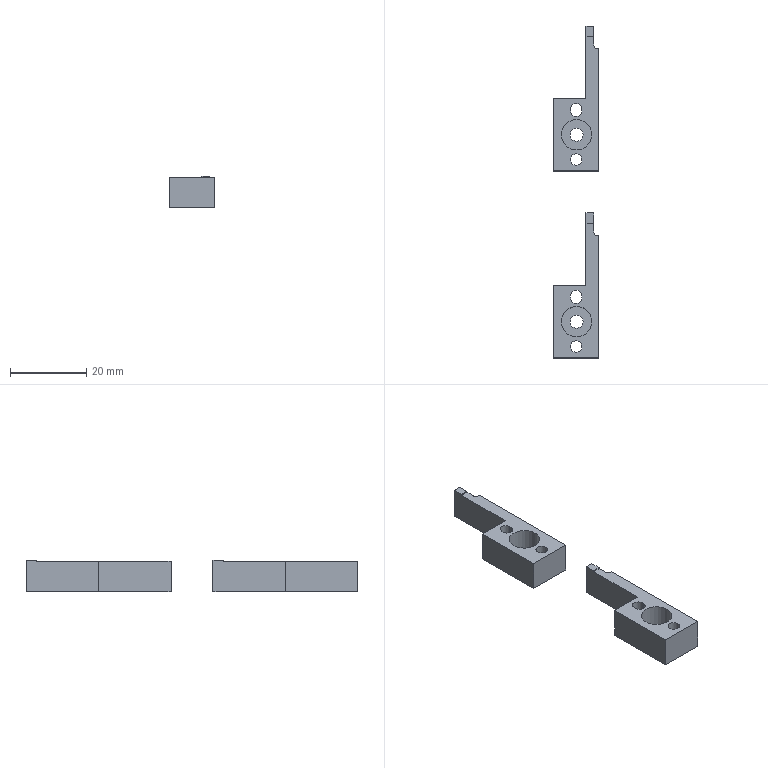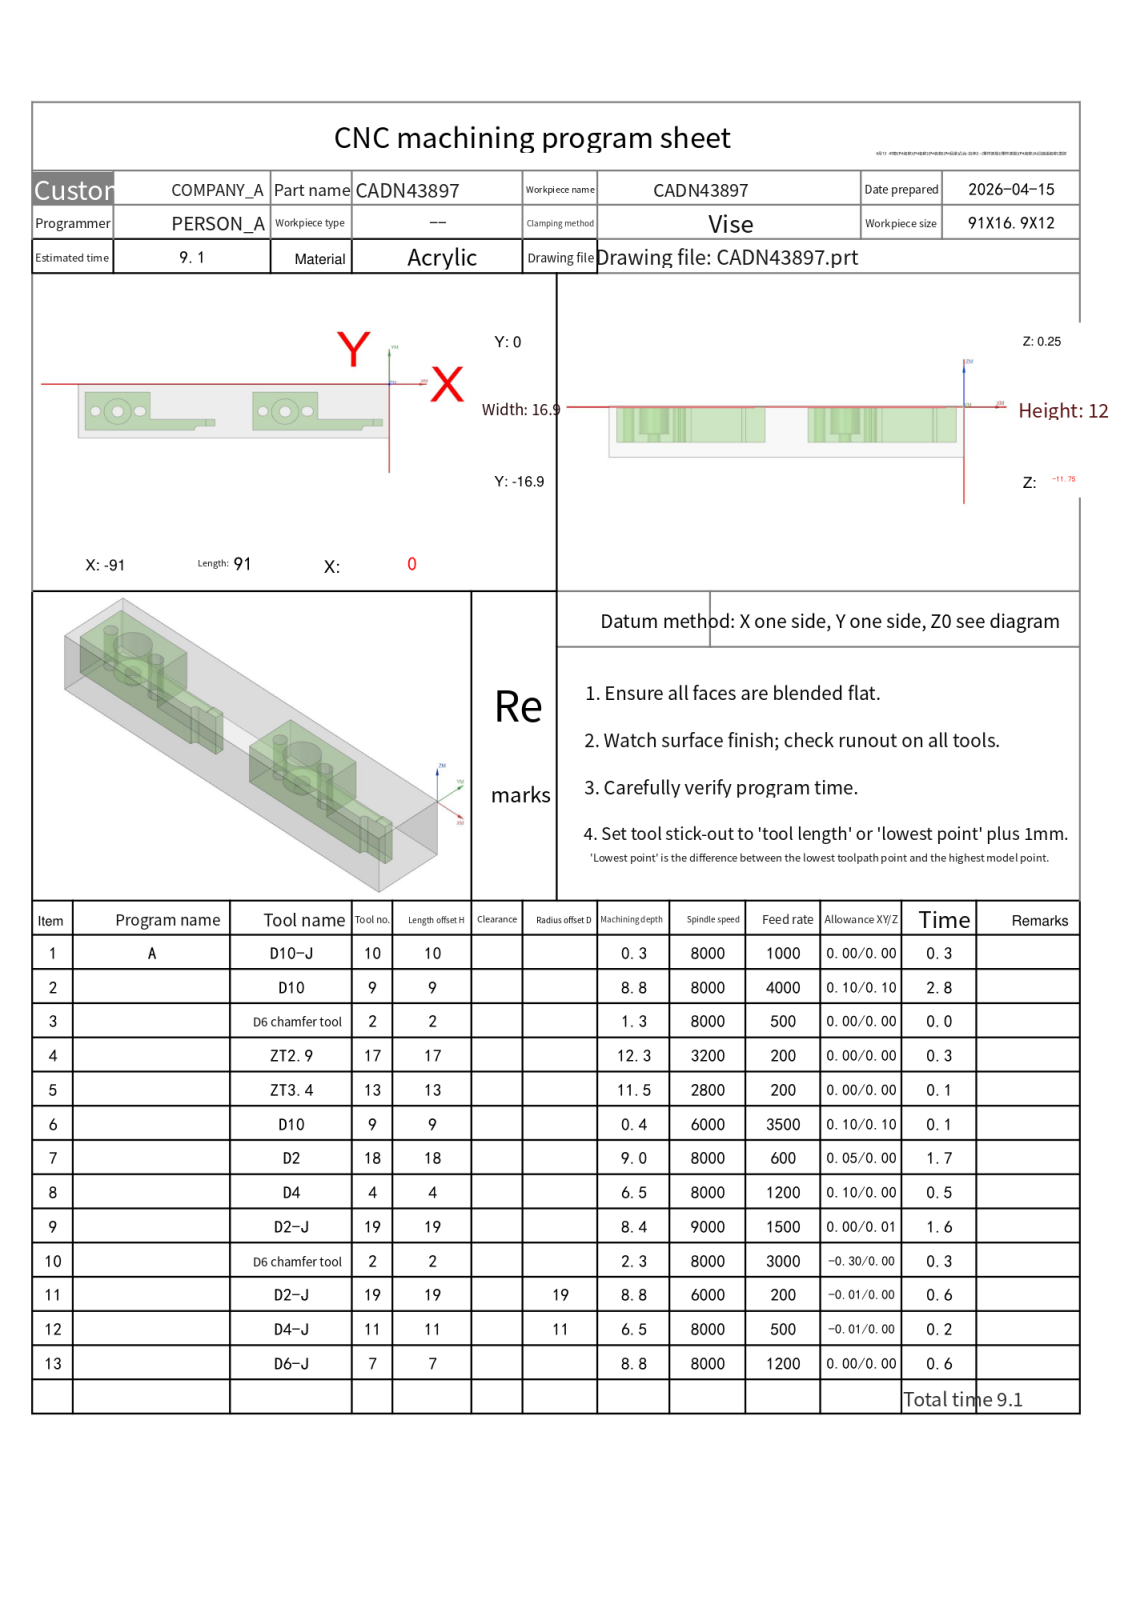NC program | NX | posted by the shop | part box 11.9 x 87 x 8.25 mm
Lines 1 to 2110 of 9110, first 1642 of 2108 lines:
%
O0001
(Machine time: 11.64 MIN)
(===Total Tool:10===)
(T10=D10-J  D=10.  R=0.   D-  H10 Z=-0.   )
(T9=D10     D=10.  R=0.   D-  H09 Z=-8.55 )
(T2=D6 chamfer tool   D=6.   R=0.   D-  H02 Z=-2.05 )
(T17=ZT2.9  D=2.9  DR_a=120 D-  H17 Z=-12.09)
(T13=ZT3.4  D=3.4  DR_a=118 D-  H13 Z=-11.27)
(T18=D2     D=2.   R=0.   D-  H18 Z=-8.75 )
(T4=D4      D=4.   R=0.   D-  H04 Z=-6.25 )
(T19=D2-J   D=2.   R=0.   D-  H19 Z=-8.55 )
(T11=D4-J   D=4.   R=0.   D11 H11 Z=-6.25 )
(T7=D6-J    D=6.   R=0.   D7  H07 Z=-8.55 )
G80 G90 G17 G49 G40
G91 G28 Z0
M01
N1 T10 M06
(D10-J  D=10. R=0. H=10 ce=0.00 di=0.00)
G00 G90 G54 X-99. Y-2.975 M03 S8000
G43 H10 Z20.
M08
Z2.
G01 Z0.0 F1000.
X-94.
X3.
Y-8.45
X-94.
Y-13.925
X3.
X8.
Z2.
G00 Z20.
G91 G28 Z0.0
M05
M09
G91 G28 Z0.0
M01
N2 T09 M06
(D10  D=10. R=0. H=09 ce=0.10 di=0.10)
G00 G90 G54 X-62.25 Y12. M03 S8000
G43 H09 Z10.25
M08
Z.725
G01 Z-.475 F4000.
Y7.5
G03 X-55.25 Y.5 I7. J0.0
G01 X-45.766
G02 X-40. Y4. I5.766 J-3.
G01 X-21.
G02 X-15.234 Y.5 I0.0 J-6.5
G01 X0.0
G02 X.5 Y0.0 I0.0 J-.5
G01 Y-4.341
G02 X-.5 Y-5.341 I-1. J0.0
X-.786 Y-5.299 I0.0 J1.
G01 X-3.474 Y-4.498
G03 X-3.76 Y-4.456 I-.285 J-.958
X-4.126 Y-4.526 I0.0 J-1.
G01 X-4.199 Y-4.54
X-14.301
G02 X-14.5 Y-4.341 I.001 J.2
G01 Y-4.199
G02 X-14.301 Y-4. I.2 J-.001
G01 X-4.199
X-4.121 Y-4.016
G03 X-3.726 Y-4.098 I.395 J.919
X-3.48 Y-4.067 I0.0 J1.
G01 X-.746 Y-3.372
G02 X-.5 Y-3.341 I.246 J-.969
X.5 Y-4.341 I0.0 J-1.
G01 Y-5.04
G02 X4.5 Y-11.04 I-2.5 J-6.
G01 Y-13.1
G02 X-2. Y-19.6 I-6.5 J0.0
G01 X-4.1
G02 X-8. Y-20.9 I-3.9 J5.2
G01 X-40.
G02 X-45.766 Y-17.4 I0.0 J6.5
G01 X-46.126
G02 X-51. Y-19.6 I-4.874 J4.3
G01 X-53.1
G02 X-57. Y-20.9 I-3.9 J5.2
G01 X-89.
G02 X-95.5 Y-14.4 I0.0 J6.5
G01 Y-2.5
G02 X-89. Y4. I6.5 J0.0
G01 X-70.
G02 X-64.234 Y.5 I0.0 J-6.5
G01 X-50.25
G02 X-49.26 Y-.357 I0.0 J-1.
G01 X-48.912 Y-2.774
G03 X-47.496 Y-4. I1.416 J.204
G01 X-47.198
G02 X-46.513 Y-4.568 I-.002 J-.7
G03 X-46.082 Y-5.125 I.765 J.147
G01 X-45.7 Y-5.306
X-45.52 Y-5.346
G03 X-45.1 Y-4.926 I0.0 J.42
G01 Y-2.5
G02 X-40. Y2.6 I5.1 J0.0
G01 X-21.
G02 X-15.9 Y-2.5 I0.0 J-5.1
G01 Y-5.94
X-2.
G02 X3.1 Y-11.04 I0.0 J-5.1
G01 Y-13.1
G02 X-2. Y-18.2 I-5.1 J0.0
G01 X-4.599
G02 X-8. Y-19.5 I-3.401 J3.8
G01 X-40.
G02 X-45.1 Y-14.4 I0.0 J5.1
G01 Y-4.926
G03 X-45.52 Y-4.506 I-.42 J0.0
G01 X-45.7 Y-4.547
X-46.306 Y-4.834
G03 X-46.522 Y-5.097 I.172 J-.361
G02 X-47.2 Y-5.624 I-.678 J.172
X-47.568 Y-5.52 I0.0 J.7
G03 X-51. Y-4.54 I-3.432 J-5.52
G01 X-63.301
G02 X-63.481 Y-4.425 I.001 J.2
G03 X-63.892 Y-4.013 I-.783 J-.37
G01 X-64.3 Y-3.819
X-64.48 Y-3.779
G03 X-64.9 Y-4.199 I0.0 J-.42
G01 Y-5.94
X-51.
G02 X-45.9 Y-11.04 I0.0 J-5.1
G01 Y-13.1
G02 X-51. Y-18.2 I-5.1 J0.0
G01 X-53.599
G02 X-57. Y-19.5 I-3.401 J3.8
G01 X-89.
G02 X-94.1 Y-14.4 I0.0 J5.1
G01 Y-2.5
G02 X-89. Y2.6 I5.1 J0.0
G01 X-70.
G02 X-64.9 Y-2.5 I0.0 J-5.1
G01 Y-4.199
G03 X-64.48 Y-4.619 I.42 J0.0
G01 X-64.3 Y-4.578
X-63.654 Y-4.272
G03 X-63.475 Y-4.104 I-.172 J.361
G02 X-63.301 Y-4. I.175 J-.096
G01 X-50.25
X-49.75
G03 X-46.25 Y-.5 I0.0 J3.5
G01 Y12.
Z.725
G00 Z3.
G01 X-62.25 F6000.
G00 Z.25
G01 Z-.95 F4000.
Y7.5
G03 X-55.25 Y.5 I7. J0.0
G01 X-45.766
G02 X-40. Y4. I5.766 J-3.
G01 X-21.
G02 X-15.234 Y.5 I0.0 J-6.5
G01 X0.0
G02 X.5 Y0.0 I0.0 J-.5
G01 Y-4.341
G02 X-.5 Y-5.341 I-1. J0.0
X-.786 Y-5.299 I0.0 J1.
G01 X-3.474 Y-4.498
G03 X-3.759 Y-4.456 I-.285 J-.958
X-4.126 Y-4.526 I0.0 J-1.
G01 X-4.199 Y-4.54
X-14.301
G02 X-14.5 Y-4.341 I.001 J.2
G01 Y-4.199
G02 X-14.301 Y-4. I.2 J-.001
G01 X-4.199
X-4.121 Y-4.016
G03 X-3.726 Y-4.098 I.395 J.919
X-3.48 Y-4.067 I0.0 J1.
G01 X-.746 Y-3.372
G02 X-.5 Y-3.341 I.246 J-.969
X.5 Y-4.341 I0.0 J-1.
G01 Y-5.04
G02 X4.5 Y-11.04 I-2.5 J-6.
G01 Y-13.1
G02 X-2. Y-19.6 I-6.5 J0.0
G01 X-4.1
G02 X-8. Y-20.9 I-3.9 J5.2
G01 X-40.
G02 X-45.766 Y-17.4 I0.0 J6.5
G01 X-46.126
G02 X-51. Y-19.6 I-4.874 J4.3
G01 X-53.1
G02 X-57. Y-20.9 I-3.9 J5.2
G01 X-89.
G02 X-95.5 Y-14.4 I0.0 J6.5
G01 Y-2.5
G02 X-89. Y4. I6.5 J0.0
G01 X-70.
G02 X-64.234 Y.5 I0.0 J-6.5
G01 X-50.25
G02 X-49.26 Y-.357 I0.0 J-1.
G01 X-48.912 Y-2.774
G03 X-47.496 Y-4. I1.416 J.204
G01 X-47.198
G02 X-46.513 Y-4.568 I-.002 J-.7
G03 X-46.082 Y-5.125 I.765 J.147
G01 X-45.7 Y-5.306
X-45.52 Y-5.346
G03 X-45.1 Y-4.926 I0.0 J.42
G01 Y-2.5
G02 X-40. Y2.6 I5.1 J0.0
G01 X-21.
G02 X-15.9 Y-2.5 I0.0 J-5.1
G01 Y-5.94
X-2.
G02 X3.1 Y-11.04 I0.0 J-5.1
G01 Y-13.1
G02 X-2. Y-18.2 I-5.1 J0.0
G01 X-4.599
G02 X-8. Y-19.5 I-3.401 J3.8
G01 X-40.
G02 X-45.1 Y-14.4 I0.0 J5.1
G01 Y-4.926
G03 X-45.52 Y-4.506 I-.42 J0.0
G01 X-45.7 Y-4.547
X-46.305 Y-4.834
G03 X-46.521 Y-5.097 I.172 J-.361
G02 X-47.2 Y-5.624 I-.678 J.172
X-47.568 Y-5.52 I0.0 J.7
G03 X-51. Y-4.54 I-3.432 J-5.52
G01 X-63.301
G02 X-63.481 Y-4.425 I.001 J.2
G03 X-63.892 Y-4.013 I-.783 J-.37
G01 X-64.3 Y-3.82
X-64.48 Y-3.779
G03 X-64.9 Y-4.199 I0.0 J-.42
G01 Y-5.94
X-51.
G02 X-45.9 Y-11.04 I0.0 J-5.1
G01 Y-13.1
G02 X-51. Y-18.2 I-5.1 J0.0
G01 X-53.599
G02 X-57. Y-19.5 I-3.401 J3.8
G01 X-89.
G02 X-94.1 Y-14.4 I0.0 J5.1
G01 Y-2.5
G02 X-89. Y2.6 I5.1 J0.0
G01 X-70.
G02 X-64.9 Y-2.5 I0.0 J-5.1
G01 Y-4.199
G03 X-64.48 Y-4.619 I.42 J0.0
G01 X-64.3 Y-4.579
X-63.654 Y-4.272
G03 X-63.475 Y-4.104 I-.172 J.361
G02 X-63.301 Y-4. I.175 J-.096
G01 X-50.25
X-49.75
G03 X-46.25 Y-.5 I0.0 J3.5
G01 Y12.
Z.25
G00 Z2.525
G01 X-62.25 F6000.
G00 Z-.225
G01 Z-1.425 F4000.
Y7.5
G03 X-55.25 Y.5 I7. J0.0
G01 X-45.766
G02 X-40. Y4. I5.766 J-3.
G01 X-21.
G02 X-15.234 Y.5 I0.0 J-6.5
G01 X0.0
G02 X.5 Y0.0 I0.0 J-.5
G01 Y-4.341
G02 X-.5 Y-5.341 I-1. J0.0
X-.786 Y-5.299 I0.0 J1.
G01 X-3.474 Y-4.498
G03 X-3.76 Y-4.456 I-.285 J-.958
X-4.126 Y-4.526 I0.0 J-1.
G01 X-4.199 Y-4.54
X-14.301
G02 X-14.5 Y-4.341 I.001 J.2
G01 Y-4.199
G02 X-14.301 Y-4. I.2 J-.001
G01 X-4.199
X-4.121 Y-4.016
G03 X-3.726 Y-4.098 I.395 J.919
X-3.48 Y-4.067 I0.0 J1.
G01 X-.746 Y-3.372
G02 X-.5 Y-3.341 I.246 J-.969
X.5 Y-4.341 I0.0 J-1.
G01 Y-5.04
G02 X4.5 Y-11.04 I-2.5 J-6.
G01 Y-13.1
G02 X-2. Y-19.6 I-6.5 J0.0
G01 X-4.1
G02 X-8. Y-20.9 I-3.9 J5.2
G01 X-40.
G02 X-45.766 Y-17.4 I0.0 J6.5
G01 X-46.126
G02 X-51. Y-19.6 I-4.874 J4.3
G01 X-53.1
G02 X-57. Y-20.9 I-3.9 J5.2
G01 X-89.
G02 X-95.5 Y-14.4 I0.0 J6.5
G01 Y-2.5
G02 X-89. Y4. I6.5 J0.0
G01 X-70.
G02 X-64.234 Y.5 I0.0 J-6.5
G01 X-50.25
G02 X-49.26 Y-.357 I0.0 J-1.
G01 X-48.912 Y-2.774
G03 X-47.496 Y-4. I1.416 J.204
G01 X-47.198
G02 X-46.513 Y-4.568 I-.002 J-.7
G03 X-46.082 Y-5.125 I.765 J.147
G01 X-45.7 Y-5.306
X-45.52 Y-5.346
G03 X-45.1 Y-4.926 I0.0 J.42
G01 Y-2.5
G02 X-40. Y2.6 I5.1 J0.0
G01 X-21.
G02 X-15.9 Y-2.5 I0.0 J-5.1
G01 Y-5.94
X-2.
G02 X3.1 Y-11.04 I0.0 J-5.1
G01 Y-13.1
G02 X-2. Y-18.2 I-5.1 J0.0
G01 X-4.599
G02 X-8. Y-19.5 I-3.401 J3.8
G01 X-40.
G02 X-45.1 Y-14.4 I0.0 J5.1
G01 Y-4.926
G03 X-45.52 Y-4.506 I-.42 J0.0
G01 X-45.7 Y-4.547
X-46.306 Y-4.834
G03 X-46.522 Y-5.097 I.172 J-.361
G02 X-47.2 Y-5.624 I-.678 J.172
X-47.568 Y-5.52 I0.0 J.7
G03 X-51. Y-4.54 I-3.432 J-5.52
G01 X-63.301
G02 X-63.481 Y-4.425 I.001 J.2
G03 X-63.892 Y-4.013 I-.783 J-.37
G01 X-64.3 Y-3.819
X-64.48 Y-3.779
G03 X-64.9 Y-4.199 I0.0 J-.42
G01 Y-5.94
X-51.
G02 X-45.9 Y-11.04 I0.0 J-5.1
G01 Y-13.1
G02 X-51. Y-18.2 I-5.1 J0.0
G01 X-53.599
G02 X-57. Y-19.5 I-3.401 J3.8
G01 X-89.
G02 X-94.1 Y-14.4 I0.0 J5.1
G01 Y-2.5
G02 X-89. Y2.6 I5.1 J0.0
G01 X-70.
G02 X-64.9 Y-2.5 I0.0 J-5.1
G01 Y-4.199
G03 X-64.48 Y-4.619 I.42 J0.0
G01 X-64.3 Y-4.578
X-63.654 Y-4.272
G03 X-63.475 Y-4.104 I-.172 J.361
G02 X-63.301 Y-4. I.175 J-.096
G01 X-50.25
X-49.75
G03 X-46.25 Y-.5 I0.0 J3.5
G01 Y12.
Z-.225
G00 Z2.05
G01 X-62.25 F6000.
G00 Z-.7
G01 Z-1.9 F4000.
Y7.5
G03 X-55.25 Y.5 I7. J0.0
G01 X-45.766
G02 X-40. Y4. I5.766 J-3.
G01 X-21.
G02 X-15.234 Y.5 I0.0 J-6.5
G01 X0.0
G02 X.5 Y0.0 I0.0 J-.5
G01 Y-4.341
G02 X-.5 Y-5.341 I-1. J0.0
X-.786 Y-5.299 I0.0 J1.
G01 X-3.474 Y-4.498
G03 X-3.759 Y-4.456 I-.285 J-.958
X-4.126 Y-4.526 I0.0 J-1.
G01 X-4.199 Y-4.54
X-14.301
G02 X-14.5 Y-4.341 I.001 J.2
G01 Y-4.199
G02 X-14.301 Y-4. I.2 J-.001
G01 X-4.199
X-4.121 Y-4.016
G03 X-3.726 Y-4.098 I.395 J.919
X-3.48 Y-4.067 I0.0 J1.
G01 X-.746 Y-3.372
G02 X-.5 Y-3.341 I.246 J-.969
X.5 Y-4.341 I0.0 J-1.
G01 Y-5.04
G02 X4.5 Y-11.04 I-2.5 J-6.
G01 Y-13.1
G02 X-2. Y-19.6 I-6.5 J0.0
G01 X-4.1
G02 X-8. Y-20.9 I-3.9 J5.2
G01 X-40.
G02 X-45.766 Y-17.4 I0.0 J6.5
G01 X-46.126
G02 X-51. Y-19.6 I-4.874 J4.3
G01 X-53.1
G02 X-57. Y-20.9 I-3.9 J5.2
G01 X-89.
G02 X-95.5 Y-14.4 I0.0 J6.5
G01 Y-2.5
G02 X-89. Y4. I6.5 J0.0
G01 X-70.
G02 X-64.234 Y.5 I0.0 J-6.5
G01 X-50.25
G02 X-49.26 Y-.357 I0.0 J-1.
G01 X-48.912 Y-2.774
G03 X-47.496 Y-4. I1.416 J.204
G01 X-47.198
G02 X-46.513 Y-4.568 I-.002 J-.7
G03 X-46.082 Y-5.125 I.765 J.147
G01 X-45.7 Y-5.306
X-45.52 Y-5.346
G03 X-45.1 Y-4.926 I0.0 J.42
G01 Y-2.5
G02 X-40. Y2.6 I5.1 J0.0
G01 X-21.
G02 X-15.9 Y-2.5 I0.0 J-5.1
G01 Y-5.94
X-2.
G02 X3.1 Y-11.04 I0.0 J-5.1
G01 Y-13.1
G02 X-2. Y-18.2 I-5.1 J0.0
G01 X-4.599
G02 X-8. Y-19.5 I-3.401 J3.8
G01 X-40.
G02 X-45.1 Y-14.4 I0.0 J5.1
G01 Y-4.926
G03 X-45.52 Y-4.506 I-.42 J0.0
G01 X-45.7 Y-4.547
X-46.305 Y-4.834
G03 X-46.521 Y-5.097 I.172 J-.361
G02 X-47.2 Y-5.624 I-.678 J.172
X-47.568 Y-5.52 I0.0 J.7
G03 X-51. Y-4.54 I-3.432 J-5.52
G01 X-63.301
G02 X-63.481 Y-4.425 I.001 J.2
G03 X-63.892 Y-4.013 I-.783 J-.37
G01 X-64.3 Y-3.82
X-64.48 Y-3.779
G03 X-64.9 Y-4.199 I0.0 J-.42
G01 Y-5.94
X-51.
G02 X-45.9 Y-11.04 I0.0 J-5.1
G01 Y-13.1
G02 X-51. Y-18.2 I-5.1 J0.0
G01 X-53.599
G02 X-57. Y-19.5 I-3.401 J3.8
G01 X-89.
G02 X-94.1 Y-14.4 I0.0 J5.1
G01 Y-2.5
G02 X-89. Y2.6 I5.1 J0.0
G01 X-70.
G02 X-64.9 Y-2.5 I0.0 J-5.1
G01 Y-4.199
G03 X-64.48 Y-4.619 I.42 J0.0
G01 X-64.3 Y-4.579
X-63.654 Y-4.272
G03 X-63.475 Y-4.104 I-.172 J.361
G02 X-63.301 Y-4. I.175 J-.096
G01 X-50.25
X-49.75
G03 X-46.25 Y-.5 I0.0 J3.5
G01 Y12.
Z-.7
G00 Z1.575
G01 X-62.25 F6000.
G00 Z-1.175
G01 Z-2.375 F4000.
Y7.5
G03 X-55.25 Y.5 I7. J0.0
G01 X-45.766
G02 X-40. Y4. I5.766 J-3.
G01 X-21.
G02 X-15.234 Y.5 I0.0 J-6.5
G01 X0.0
G02 X.5 Y0.0 I0.0 J-.5
G01 Y-4.341
G02 X-.5 Y-5.341 I-1. J0.0
X-.786 Y-5.299 I0.0 J1.
G01 X-3.474 Y-4.498
G03 X-3.76 Y-4.456 I-.285 J-.958
X-4.126 Y-4.526 I0.0 J-1.
G01 X-4.199 Y-4.54
X-14.301
G02 X-14.5 Y-4.341 I.001 J.2
G01 Y-4.199
G02 X-14.301 Y-4. I.2 J-.001
G01 X-4.199
X-4.121 Y-4.016
G03 X-3.726 Y-4.098 I.395 J.919
X-3.48 Y-4.067 I0.0 J1.
G01 X-.746 Y-3.372
G02 X-.5 Y-3.341 I.246 J-.969
X.5 Y-4.341 I0.0 J-1.
G01 Y-5.04
G02 X4.5 Y-11.04 I-2.5 J-6.
G01 Y-13.1
G02 X-2. Y-19.6 I-6.5 J0.0
G01 X-4.1
G02 X-8. Y-20.9 I-3.9 J5.2
G01 X-40.
G02 X-45.766 Y-17.4 I0.0 J6.5
G01 X-46.126
G02 X-51. Y-19.6 I-4.874 J4.3
G01 X-53.1
G02 X-57. Y-20.9 I-3.9 J5.2
G01 X-89.
G02 X-95.5 Y-14.4 I0.0 J6.5
G01 Y-2.5
G02 X-89. Y4. I6.5 J0.0
G01 X-70.
G02 X-64.234 Y.5 I0.0 J-6.5
G01 X-50.25
G02 X-49.26 Y-.357 I0.0 J-1.
G01 X-48.912 Y-2.774
G03 X-47.496 Y-4. I1.416 J.204
G01 X-47.198
G02 X-46.513 Y-4.568 I-.002 J-.7
G03 X-46.082 Y-5.125 I.765 J.147
G01 X-45.7 Y-5.306
X-45.52 Y-5.346
G03 X-45.1 Y-4.926 I0.0 J.42
G01 Y-2.5
G02 X-40. Y2.6 I5.1 J0.0
G01 X-21.
G02 X-15.9 Y-2.5 I0.0 J-5.1
G01 Y-5.94
X-2.
G02 X3.1 Y-11.04 I0.0 J-5.1
G01 Y-13.1
G02 X-2. Y-18.2 I-5.1 J0.0
G01 X-4.599
G02 X-8. Y-19.5 I-3.401 J3.8
G01 X-40.
G02 X-45.1 Y-14.4 I0.0 J5.1
G01 Y-4.926
G03 X-45.52 Y-4.506 I-.42 J0.0
G01 X-45.7 Y-4.547
X-46.306 Y-4.834
G03 X-46.522 Y-5.097 I.172 J-.361
G02 X-47.2 Y-5.624 I-.678 J.172
X-47.568 Y-5.52 I0.0 J.7
G03 X-51. Y-4.54 I-3.432 J-5.52
G01 X-63.301
G02 X-63.481 Y-4.425 I.001 J.2
G03 X-63.892 Y-4.013 I-.783 J-.37
G01 X-64.3 Y-3.819
X-64.48 Y-3.779
G03 X-64.9 Y-4.199 I0.0 J-.42
G01 Y-5.94
X-51.
G02 X-45.9 Y-11.04 I0.0 J-5.1
G01 Y-13.1
G02 X-51. Y-18.2 I-5.1 J0.0
G01 X-53.599
G02 X-57. Y-19.5 I-3.401 J3.8
G01 X-89.
G02 X-94.1 Y-14.4 I0.0 J5.1
G01 Y-2.5
G02 X-89. Y2.6 I5.1 J0.0
G01 X-70.
G02 X-64.9 Y-2.5 I0.0 J-5.1
G01 Y-4.199
G03 X-64.48 Y-4.619 I.42 J0.0
G01 X-64.3 Y-4.578
X-63.654 Y-4.272
G03 X-63.475 Y-4.104 I-.172 J.361
G02 X-63.301 Y-4. I.175 J-.096
G01 X-50.25
X-49.75
G03 X-46.25 Y-.5 I0.0 J3.5
G01 Y12.
Z-1.175
G00 Z1.1
G01 X-62.25 F6000.
G00 Z-1.65
G01 Z-2.85 F4000.
Y7.5
G03 X-55.25 Y.5 I7. J0.0
G01 X-45.766
G02 X-40. Y4. I5.766 J-3.
G01 X-21.
G02 X-15.234 Y.5 I0.0 J-6.5
G01 X0.0
G02 X.5 Y0.0 I0.0 J-.5
G01 Y-4.341
G02 X-.5 Y-5.341 I-1. J0.0
X-.786 Y-5.299 I0.0 J1.
G01 X-3.474 Y-4.498
G03 X-3.759 Y-4.456 I-.285 J-.958
X-4.126 Y-4.526 I0.0 J-1.
G01 X-4.199 Y-4.54
X-14.301
G02 X-14.5 Y-4.341 I.001 J.2
G01 Y-4.199
G02 X-14.301 Y-4. I.2 J-.001
G01 X-4.199
X-4.121 Y-4.016
G03 X-3.726 Y-4.098 I.395 J.919
X-3.48 Y-4.067 I0.0 J1.
G01 X-.746 Y-3.372
G02 X-.5 Y-3.341 I.246 J-.969
X.5 Y-4.341 I0.0 J-1.
G01 Y-5.04
G02 X4.5 Y-11.04 I-2.5 J-6.
G01 Y-13.1
G02 X-2. Y-19.6 I-6.5 J0.0
G01 X-4.1
G02 X-8. Y-20.9 I-3.9 J5.2
G01 X-40.
G02 X-45.766 Y-17.4 I0.0 J6.5
G01 X-46.126
G02 X-51. Y-19.6 I-4.874 J4.3
G01 X-53.1
G02 X-57. Y-20.9 I-3.9 J5.2
G01 X-89.
G02 X-95.5 Y-14.4 I0.0 J6.5
G01 Y-2.5
G02 X-89. Y4. I6.5 J0.0
G01 X-70.
G02 X-64.234 Y.5 I0.0 J-6.5
G01 X-50.25
G02 X-49.26 Y-.357 I0.0 J-1.
G01 X-48.912 Y-2.774
G03 X-47.496 Y-4. I1.416 J.204
G01 X-47.198
G02 X-46.513 Y-4.568 I-.002 J-.7
G03 X-46.082 Y-5.125 I.765 J.147
G01 X-45.7 Y-5.306
X-45.52 Y-5.346
G03 X-45.1 Y-4.926 I0.0 J.42
G01 Y-2.5
G02 X-40. Y2.6 I5.1 J0.0
G01 X-21.
G02 X-15.9 Y-2.5 I0.0 J-5.1
G01 Y-5.94
X-2.
G02 X3.1 Y-11.04 I0.0 J-5.1
G01 Y-13.1
G02 X-2. Y-18.2 I-5.1 J0.0
G01 X-4.599
G02 X-8. Y-19.5 I-3.401 J3.8
G01 X-40.
G02 X-45.1 Y-14.4 I0.0 J5.1
G01 Y-4.926
G03 X-45.52 Y-4.506 I-.42 J0.0
G01 X-45.7 Y-4.547
X-46.305 Y-4.834
G03 X-46.521 Y-5.097 I.172 J-.361
G02 X-47.2 Y-5.624 I-.678 J.172
X-47.568 Y-5.52 I0.0 J.7
G03 X-51. Y-4.54 I-3.432 J-5.52
G01 X-63.301
G02 X-63.481 Y-4.425 I.001 J.2
G03 X-63.892 Y-4.013 I-.783 J-.37
G01 X-64.3 Y-3.82
X-64.48 Y-3.779
G03 X-64.9 Y-4.199 I0.0 J-.42
G01 Y-5.94
X-51.
G02 X-45.9 Y-11.04 I0.0 J-5.1
G01 Y-13.1
G02 X-51. Y-18.2 I-5.1 J0.0
G01 X-53.599
G02 X-57. Y-19.5 I-3.401 J3.8
G01 X-89.
G02 X-94.1 Y-14.4 I0.0 J5.1
G01 Y-2.5
G02 X-89. Y2.6 I5.1 J0.0
G01 X-70.
G02 X-64.9 Y-2.5 I0.0 J-5.1
G01 Y-4.199
G03 X-64.48 Y-4.619 I.42 J0.0
G01 X-64.3 Y-4.579
X-63.654 Y-4.272
G03 X-63.475 Y-4.104 I-.172 J.361
G02 X-63.301 Y-4. I.175 J-.096
G01 X-50.25
X-49.75
G03 X-46.25 Y-.5 I0.0 J3.5
G01 Y12.
Z-1.65
G00 Z.625
G01 X-62.25 F6000.
G00 Z-2.125
G01 Z-3.325 F4000.
Y7.5
G03 X-55.25 Y.5 I7. J0.0
G01 X-45.766
G02 X-40. Y4. I5.766 J-3.
G01 X-21.
G02 X-15.234 Y.5 I0.0 J-6.5
G01 X0.0
G02 X.5 Y0.0 I0.0 J-.5
G01 Y-4.341
G02 X-.5 Y-5.341 I-1. J0.0
X-.786 Y-5.299 I0.0 J1.
G01 X-3.474 Y-4.498
G03 X-3.76 Y-4.456 I-.285 J-.958
X-4.126 Y-4.526 I0.0 J-1.
G01 X-4.199 Y-4.54
X-14.301
G02 X-14.5 Y-4.341 I.001 J.2
G01 Y-4.199
G02 X-14.301 Y-4. I.2 J-.001
G01 X-4.199
X-4.121 Y-4.016
G03 X-3.726 Y-4.098 I.395 J.919
X-3.48 Y-4.067 I0.0 J1.
G01 X-.746 Y-3.372
G02 X-.5 Y-3.341 I.246 J-.969
X.5 Y-4.341 I0.0 J-1.
G01 Y-5.04
G02 X4.5 Y-11.04 I-2.5 J-6.
G01 Y-13.1
G02 X-2. Y-19.6 I-6.5 J0.0
G01 X-4.1
G02 X-8. Y-20.9 I-3.9 J5.2
G01 X-40.
G02 X-45.766 Y-17.4 I0.0 J6.5
G01 X-46.126
G02 X-51. Y-19.6 I-4.874 J4.3
G01 X-53.1
G02 X-57. Y-20.9 I-3.9 J5.2
G01 X-89.
G02 X-95.5 Y-14.4 I0.0 J6.5
G01 Y-2.5
G02 X-89. Y4. I6.5 J0.0
G01 X-70.
G02 X-64.234 Y.5 I0.0 J-6.5
G01 X-50.25
G02 X-49.26 Y-.357 I0.0 J-1.
G01 X-48.912 Y-2.774
G03 X-47.496 Y-4. I1.416 J.204
G01 X-47.198
G02 X-46.513 Y-4.568 I-.002 J-.7
G03 X-46.082 Y-5.125 I.765 J.147
G01 X-45.7 Y-5.306
X-45.52 Y-5.346
G03 X-45.1 Y-4.926 I0.0 J.42
G01 Y-2.5
G02 X-40. Y2.6 I5.1 J0.0
G01 X-21.
G02 X-15.9 Y-2.5 I0.0 J-5.1
G01 Y-5.94
X-2.
G02 X3.1 Y-11.04 I0.0 J-5.1
G01 Y-13.1
G02 X-2. Y-18.2 I-5.1 J0.0
G01 X-4.599
G02 X-8. Y-19.5 I-3.401 J3.8
G01 X-40.
G02 X-45.1 Y-14.4 I0.0 J5.1
G01 Y-4.926
G03 X-45.52 Y-4.506 I-.42 J0.0
G01 X-45.7 Y-4.547
X-46.306 Y-4.834
G03 X-46.522 Y-5.097 I.172 J-.361
G02 X-47.2 Y-5.624 I-.678 J.172
X-47.568 Y-5.52 I0.0 J.7
G03 X-51. Y-4.54 I-3.432 J-5.52
G01 X-63.301
G02 X-63.481 Y-4.425 I.001 J.2
G03 X-63.892 Y-4.013 I-.783 J-.37
G01 X-64.3 Y-3.819
X-64.48 Y-3.779
G03 X-64.9 Y-4.199 I0.0 J-.42
G01 Y-5.94
X-51.
G02 X-45.9 Y-11.04 I0.0 J-5.1
G01 Y-13.1
G02 X-51. Y-18.2 I-5.1 J0.0
G01 X-53.599
G02 X-57. Y-19.5 I-3.401 J3.8
G01 X-89.
G02 X-94.1 Y-14.4 I0.0 J5.1
G01 Y-2.5
G02 X-89. Y2.6 I5.1 J0.0
G01 X-70.
G02 X-64.9 Y-2.5 I0.0 J-5.1
G01 Y-4.199
G03 X-64.48 Y-4.619 I.42 J0.0
G01 X-64.3 Y-4.578
X-63.654 Y-4.272
G03 X-63.475 Y-4.104 I-.172 J.361
G02 X-63.301 Y-4. I.175 J-.096
G01 X-50.25
X-49.75
G03 X-46.25 Y-.5 I0.0 J3.5
G01 Y12.
Z-2.125
G00 Z.15
G01 X-62.25 F6000.
G00 Z-2.6
G01 Z-3.8 F4000.
Y7.5
G03 X-55.25 Y.5 I7. J0.0
G01 X-45.766
G02 X-40. Y4. I5.766 J-3.
G01 X-21.
G02 X-15.234 Y.5 I0.0 J-6.5
G01 X0.0
G02 X.5 Y0.0 I0.0 J-.5
G01 Y-4.341
G02 X-.5 Y-5.341 I-1. J0.0
X-.786 Y-5.299 I0.0 J1.
G01 X-3.474 Y-4.498
G03 X-3.759 Y-4.456 I-.285 J-.958
X-4.126 Y-4.526 I0.0 J-1.
G01 X-4.199 Y-4.54
X-14.301
G02 X-14.5 Y-4.341 I.001 J.2
G01 Y-4.199
G02 X-14.301 Y-4. I.2 J-.001
G01 X-4.199
X-4.121 Y-4.016
G03 X-3.726 Y-4.098 I.395 J.919
X-3.48 Y-4.067 I0.0 J1.
G01 X-.746 Y-3.372
G02 X-.5 Y-3.341 I.246 J-.969
X.5 Y-4.341 I0.0 J-1.
G01 Y-5.04
G02 X4.5 Y-11.04 I-2.5 J-6.
G01 Y-13.1
G02 X-2. Y-19.6 I-6.5 J0.0
G01 X-4.1
G02 X-8. Y-20.9 I-3.9 J5.2
G01 X-40.
G02 X-45.766 Y-17.4 I0.0 J6.5
G01 X-46.126
G02 X-51. Y-19.6 I-4.874 J4.3
G01 X-53.1
G02 X-57. Y-20.9 I-3.9 J5.2
G01 X-89.
G02 X-95.5 Y-14.4 I0.0 J6.5
G01 Y-2.5
G02 X-89. Y4. I6.5 J0.0
G01 X-70.
G02 X-64.234 Y.5 I0.0 J-6.5
G01 X-50.25
G02 X-49.26 Y-.357 I0.0 J-1.
G01 X-48.912 Y-2.774
G03 X-47.496 Y-4. I1.416 J.204
G01 X-47.198
G02 X-46.513 Y-4.568 I-.002 J-.7
G03 X-46.082 Y-5.125 I.765 J.147
G01 X-45.7 Y-5.306
X-45.52 Y-5.346
G03 X-45.1 Y-4.926 I0.0 J.42
G01 Y-2.5
G02 X-40. Y2.6 I5.1 J0.0
G01 X-21.
G02 X-15.9 Y-2.5 I0.0 J-5.1
G01 Y-5.94
X-2.
G02 X3.1 Y-11.04 I0.0 J-5.1
G01 Y-13.1
G02 X-2. Y-18.2 I-5.1 J0.0
G01 X-4.599
G02 X-8. Y-19.5 I-3.401 J3.8
G01 X-40.
G02 X-45.1 Y-14.4 I0.0 J5.1
G01 Y-4.926
G03 X-45.52 Y-4.506 I-.42 J0.0
G01 X-45.7 Y-4.547
X-46.305 Y-4.834
G03 X-46.521 Y-5.097 I.172 J-.361
G02 X-47.2 Y-5.624 I-.678 J.172
X-47.568 Y-5.52 I0.0 J.7
G03 X-51. Y-4.54 I-3.432 J-5.52
G01 X-63.301
G02 X-63.481 Y-4.425 I.001 J.2
G03 X-63.892 Y-4.013 I-.783 J-.37
G01 X-64.3 Y-3.82
X-64.48 Y-3.779
G03 X-64.9 Y-4.199 I0.0 J-.42
G01 Y-5.94
X-51.
G02 X-45.9 Y-11.04 I0.0 J-5.1
G01 Y-13.1
G02 X-51. Y-18.2 I-5.1 J0.0
G01 X-53.599
G02 X-57. Y-19.5 I-3.401 J3.8
G01 X-89.
G02 X-94.1 Y-14.4 I0.0 J5.1
G01 Y-2.5
G02 X-89. Y2.6 I5.1 J0.0
G01 X-70.
G02 X-64.9 Y-2.5 I0.0 J-5.1
G01 Y-4.199
G03 X-64.48 Y-4.619 I.42 J0.0
G01 X-64.3 Y-4.579
X-63.654 Y-4.272
G03 X-63.475 Y-4.104 I-.172 J.361
G02 X-63.301 Y-4. I.175 J-.096
G01 X-50.25
X-49.75
G03 X-46.25 Y-.5 I0.0 J3.5
G01 Y12.
Z-2.6
G00 Z-.325
G01 X-62.25 F6000.
G00 Z-3.075
G01 Z-4.275 F4000.
Y7.5
G03 X-55.25 Y.5 I7. J0.0
G01 X-45.766
G02 X-40. Y4. I5.766 J-3.
G01 X-21.
G02 X-15.234 Y.5 I0.0 J-6.5
G01 X0.0
G02 X.5 Y0.0 I0.0 J-.5
G01 Y-4.341
G02 X-.5 Y-5.341 I-1. J0.0
X-.786 Y-5.299 I0.0 J1.
G01 X-3.474 Y-4.498
G03 X-3.76 Y-4.456 I-.285 J-.958
X-4.126 Y-4.526 I0.0 J-1.
G01 X-4.199 Y-4.54
X-14.301
G02 X-14.5 Y-4.341 I.001 J.2
G01 Y-4.199
G02 X-14.301 Y-4. I.2 J-.001
G01 X-4.199
X-4.121 Y-4.016
G03 X-3.726 Y-4.098 I.395 J.919
X-3.48 Y-4.067 I0.0 J1.
G01 X-.746 Y-3.372
G02 X-.5 Y-3.341 I.246 J-.969
X.5 Y-4.341 I0.0 J-1.
G01 Y-5.04
G02 X4.5 Y-11.04 I-2.5 J-6.
G01 Y-13.1
G02 X-2. Y-19.6 I-6.5 J0.0
G01 X-4.1
G02 X-8. Y-20.9 I-3.9 J5.2
G01 X-40.
G02 X-45.766 Y-17.4 I0.0 J6.5
G01 X-46.126
G02 X-51. Y-19.6 I-4.874 J4.3
G01 X-53.1
G02 X-57. Y-20.9 I-3.9 J5.2
G01 X-89.
G02 X-95.5 Y-14.4 I0.0 J6.5
G01 Y-2.5
G02 X-89. Y4. I6.5 J0.0
G01 X-70.
G02 X-64.234 Y.5 I0.0 J-6.5
G01 X-50.25
G02 X-49.26 Y-.357 I0.0 J-1.
G01 X-48.912 Y-2.774
G03 X-47.496 Y-4. I1.416 J.204
G01 X-47.198
G02 X-46.513 Y-4.568 I-.002 J-.7
G03 X-46.082 Y-5.125 I.765 J.147
G01 X-45.7 Y-5.306
X-45.52 Y-5.346
G03 X-45.1 Y-4.926 I0.0 J.42
G01 Y-2.5
G02 X-40. Y2.6 I5.1 J0.0
G01 X-21.
G02 X-15.9 Y-2.5 I0.0 J-5.1
G01 Y-5.94
X-2.
G02 X3.1 Y-11.04 I0.0 J-5.1
G01 Y-13.1
G02 X-2. Y-18.2 I-5.1 J0.0
G01 X-4.599
G02 X-8. Y-19.5 I-3.401 J3.8
G01 X-40.
G02 X-45.1 Y-14.4 I0.0 J5.1
G01 Y-4.926
G03 X-45.52 Y-4.506 I-.42 J0.0
G01 X-45.7 Y-4.547
X-46.306 Y-4.834
G03 X-46.522 Y-5.097 I.172 J-.361
G02 X-47.2 Y-5.624 I-.678 J.172
X-47.568 Y-5.52 I0.0 J.7
G03 X-51. Y-4.54 I-3.432 J-5.52
G01 X-63.301
G02 X-63.481 Y-4.425 I.001 J.2
G03 X-63.892 Y-4.013 I-.783 J-.37
G01 X-64.3 Y-3.819
X-64.48 Y-3.779
G03 X-64.9 Y-4.199 I0.0 J-.42
G01 Y-5.94
X-51.
G02 X-45.9 Y-11.04 I0.0 J-5.1
G01 Y-13.1
G02 X-51. Y-18.2 I-5.1 J0.0
G01 X-53.599
G02 X-57. Y-19.5 I-3.401 J3.8
G01 X-89.
G02 X-94.1 Y-14.4 I0.0 J5.1
G01 Y-2.5
G02 X-89. Y2.6 I5.1 J0.0
G01 X-70.
G02 X-64.9 Y-2.5 I0.0 J-5.1
G01 Y-4.199
G03 X-64.48 Y-4.619 I.42 J0.0
G01 X-64.3 Y-4.578
X-63.654 Y-4.272
G03 X-63.475 Y-4.104 I-.172 J.361
G02 X-63.301 Y-4. I.175 J-.096
G01 X-50.25
X-49.75
G03 X-46.25 Y-.5 I0.0 J3.5
G01 Y12.
Z-3.075
G00 Z-.8
G01 X-62.25 F6000.
G00 Z-3.55
G01 Z-4.75 F4000.
Y7.5
G03 X-55.25 Y.5 I7. J0.0
G01 X-45.766
G02 X-40. Y4. I5.766 J-3.
G01 X-21.
G02 X-15.234 Y.5 I0.0 J-6.5
G01 X0.0
G02 X.5 Y0.0 I0.0 J-.5
G01 Y-4.341
G02 X-.5 Y-5.341 I-1. J0.0
X-.786 Y-5.299 I0.0 J1.
G01 X-3.474 Y-4.498
G03 X-3.759 Y-4.456 I-.285 J-.958
X-4.126 Y-4.526 I0.0 J-1.
G01 X-4.199 Y-4.54
X-14.301
G02 X-14.5 Y-4.341 I.001 J.2
G01 Y-4.199
G02 X-14.301 Y-4. I.2 J-.001
G01 X-4.199
X-4.121 Y-4.016
G03 X-3.726 Y-4.098 I.395 J.919
X-3.48 Y-4.067 I0.0 J1.
G01 X-.746 Y-3.372
G02 X-.5 Y-3.341 I.246 J-.969
X.5 Y-4.341 I0.0 J-1.
G01 Y-5.04
G02 X4.5 Y-11.04 I-2.5 J-6.
G01 Y-13.1
G02 X-2. Y-19.6 I-6.5 J0.0
G01 X-4.1
G02 X-8. Y-20.9 I-3.9 J5.2
G01 X-40.
G02 X-45.766 Y-17.4 I0.0 J6.5
G01 X-46.126
G02 X-51. Y-19.6 I-4.874 J4.3
G01 X-53.1
G02 X-57. Y-20.9 I-3.9 J5.2
G01 X-89.
G02 X-95.5 Y-14.4 I0.0 J6.5
G01 Y-2.5
G02 X-89. Y4. I6.5 J0.0
G01 X-70.
G02 X-64.234 Y.5 I0.0 J-6.5
G01 X-50.25
G02 X-49.26 Y-.357 I0.0 J-1.
G01 X-48.912 Y-2.774
G03 X-47.496 Y-4. I1.416 J.204
G01 X-47.198
G02 X-46.513 Y-4.568 I-.002 J-.7
G03 X-46.082 Y-5.125 I.765 J.147
G01 X-45.7 Y-5.306
X-45.52 Y-5.346
G03 X-45.1 Y-4.926 I0.0 J.42
G01 Y-2.5
G02 X-40. Y2.6 I5.1 J0.0
G01 X-21.
G02 X-15.9 Y-2.5 I0.0 J-5.1
G01 Y-5.94
X-2.
G02 X3.1 Y-11.04 I0.0 J-5.1
G01 Y-13.1
G02 X-2. Y-18.2 I-5.1 J0.0
G01 X-4.599
G02 X-8. Y-19.5 I-3.401 J3.8
G01 X-40.
G02 X-45.1 Y-14.4 I0.0 J5.1
G01 Y-4.926
G03 X-45.52 Y-4.506 I-.42 J0.0
G01 X-45.7 Y-4.547
X-46.305 Y-4.834
G03 X-46.521 Y-5.097 I.172 J-.361
G02 X-47.2 Y-5.624 I-.678 J.172
X-47.568 Y-5.52 I0.0 J.7
G03 X-51. Y-4.54 I-3.432 J-5.52
G01 X-63.301
G02 X-63.481 Y-4.425 I.001 J.2
G03 X-63.892 Y-4.013 I-.783 J-.37
G01 X-64.3 Y-3.82
X-64.48 Y-3.779
G03 X-64.9 Y-4.199 I0.0 J-.42
G01 Y-5.94
X-51.
G02 X-45.9 Y-11.04 I0.0 J-5.1
G01 Y-13.1
G02 X-51. Y-18.2 I-5.1 J0.0
G01 X-53.599
G02 X-57. Y-19.5 I-3.401 J3.8
G01 X-89.
G02 X-94.1 Y-14.4 I0.0 J5.1
G01 Y-2.5
G02 X-89. Y2.6 I5.1 J0.0
G01 X-70.
G02 X-64.9 Y-2.5 I0.0 J-5.1
G01 Y-4.199
G03 X-64.48 Y-4.619 I.42 J0.0
G01 X-64.3 Y-4.579
X-63.654 Y-4.272
G03 X-63.475 Y-4.104 I-.172 J.361
G02 X-63.301 Y-4. I.175 J-.096
G01 X-50.25
X-49.75
G03 X-46.25 Y-.5 I0.0 J3.5
G01 Y12.
Z-3.55
G00 Z-1.275
G01 X-62.25 F6000.
G00 Z-4.025
G01 Z-5.225 F4000.
Y7.5
G03 X-55.25 Y.5 I7. J0.0
G01 X-45.766
G02 X-40. Y4. I5.766 J-3.
G01 X-21.
G02 X-15.234 Y.5 I0.0 J-6.5
G01 X0.0
G02 X.5 Y0.0 I0.0 J-.5
G01 Y-4.341
G02 X-.5 Y-5.341 I-1. J0.0
X-.786 Y-5.299 I0.0 J1.
G01 X-3.474 Y-4.498
G03 X-3.76 Y-4.456 I-.285 J-.958
X-4.126 Y-4.526 I0.0 J-1.
G01 X-4.199 Y-4.54
X-14.301
G02 X-14.5 Y-4.341 I.001 J.2
G01 Y-4.199
G02 X-14.301 Y-4. I.2 J-.001
G01 X-4.199
X-4.121 Y-4.016
G03 X-3.726 Y-4.098 I.395 J.919
X-3.48 Y-4.067 I0.0 J1.
G01 X-.746 Y-3.372
G02 X-.5 Y-3.341 I.246 J-.969
X.5 Y-4.341 I0.0 J-1.
G01 Y-5.04
G02 X4.5 Y-11.04 I-2.5 J-6.
G01 Y-13.1
G02 X-2. Y-19.6 I-6.5 J0.0
G01 X-4.1
G02 X-8. Y-20.9 I-3.9 J5.2
G01 X-40.
G02 X-45.766 Y-17.4 I0.0 J6.5
G01 X-46.126
G02 X-51. Y-19.6 I-4.874 J4.3
G01 X-53.1
G02 X-57. Y-20.9 I-3.9 J5.2
G01 X-89.
G02 X-95.5 Y-14.4 I0.0 J6.5
G01 Y-2.5
G02 X-89. Y4. I6.5 J0.0
G01 X-70.
G02 X-64.234 Y.5 I0.0 J-6.5
G01 X-50.25
G02 X-49.26 Y-.357 I0.0 J-1.
G01 X-48.912 Y-2.774
G03 X-47.496 Y-4. I1.416 J.204
G01 X-47.198
G02 X-46.513 Y-4.568 I-.002 J-.7
G03 X-46.082 Y-5.125 I.765 J.147
G01 X-45.7 Y-5.306
X-45.52 Y-5.346
G03 X-45.1 Y-4.926 I0.0 J.42
G01 Y-2.5
G02 X-40. Y2.6 I5.1 J0.0
G01 X-21.
G02 X-15.9 Y-2.5 I0.0 J-5.1
G01 Y-5.94
X-2.
G02 X3.1 Y-11.04 I0.0 J-5.1
G01 Y-13.1
G02 X-2. Y-18.2 I-5.1 J0.0
G01 X-4.599
G02 X-8. Y-19.5 I-3.401 J3.8
G01 X-40.
G02 X-45.1 Y-14.4 I0.0 J5.1
G01 Y-4.926
G03 X-45.52 Y-4.506 I-.42 J0.0
G01 X-45.7 Y-4.547
X-46.306 Y-4.834
G03 X-46.522 Y-5.097 I.172 J-.361
G02 X-47.2 Y-5.624 I-.678 J.172
X-47.568 Y-5.52 I0.0 J.7
G03 X-51. Y-4.54 I-3.432 J-5.52
G01 X-63.301
G02 X-63.481 Y-4.425 I.001 J.2
G03 X-63.892 Y-4.013 I-.783 J-.37
G01 X-64.3 Y-3.819
X-64.48 Y-3.779
G03 X-64.9 Y-4.199 I0.0 J-.42
G01 Y-5.94
X-51.
G02 X-45.9 Y-11.04 I0.0 J-5.1
G01 Y-13.1
G02 X-51. Y-18.2 I-5.1 J0.0
G01 X-53.599
G02 X-57. Y-19.5 I-3.401 J3.8
G01 X-89.
G02 X-94.1 Y-14.4 I0.0 J5.1
G01 Y-2.5
G02 X-89. Y2.6 I5.1 J0.0
G01 X-70.
G02 X-64.9 Y-2.5 I0.0 J-5.1
G01 Y-4.199
G03 X-64.48 Y-4.619 I.42 J0.0
G01 X-64.3 Y-4.578
X-63.654 Y-4.272
G03 X-63.475 Y-4.104 I-.172 J.361
G02 X-63.301 Y-4. I.175 J-.096
G01 X-50.25
X-49.75
G03 X-46.25 Y-.5 I0.0 J3.5
G01 Y12.
Z-4.025
G00 Z-1.75
G01 X-62.25 F6000.
G00 Z-4.5
G01 Z-5.7 F4000.
Y7.5
G03 X-55.25 Y.5 I7. J0.0
G01 X-45.766
G02 X-40. Y4. I5.766 J-3.
G01 X-21.
G02 X-15.234 Y.5 I0.0 J-6.5
G01 X0.0
G02 X.5 Y0.0 I0.0 J-.5
G01 Y-4.341
G02 X-.5 Y-5.341 I-1. J0.0
X-.786 Y-5.299 I0.0 J1.
G01 X-3.474 Y-4.498
G03 X-3.759 Y-4.456 I-.285 J-.958
X-4.126 Y-4.526 I0.0 J-1.
G01 X-4.199 Y-4.54
X-14.301
G02 X-14.5 Y-4.341 I.001 J.2
G01 Y-4.199
G02 X-14.301 Y-4. I.2 J-.001
G01 X-4.199
X-4.121 Y-4.016
G03 X-3.726 Y-4.098 I.395 J.919
X-3.48 Y-4.067 I0.0 J1.
G01 X-.746 Y-3.372
G02 X-.5 Y-3.341 I.246 J-.969
X.5 Y-4.341 I0.0 J-1.
G01 Y-5.04
G02 X4.5 Y-11.04 I-2.5 J-6.
G01 Y-13.1
G02 X-2. Y-19.6 I-6.5 J0.0
G01 X-4.1
G02 X-8. Y-20.9 I-3.9 J5.2
G01 X-40.
G02 X-45.766 Y-17.4 I0.0 J6.5
G01 X-46.126
G02 X-51. Y-19.6 I-4.874 J4.3
G01 X-53.1
G02 X-57. Y-20.9 I-3.9 J5.2
G01 X-89.
G02 X-95.5 Y-14.4 I0.0 J6.5
G01 Y-2.5
G02 X-89. Y4. I6.5 J0.0
G01 X-70.
G02 X-64.234 Y.5 I0.0 J-6.5
G01 X-50.25
G02 X-49.26 Y-.357 I0.0 J-1.
G01 X-48.912 Y-2.774
G03 X-47.496 Y-4. I1.416 J.204
G01 X-47.198
G02 X-46.513 Y-4.568 I-.002 J-.7
G03 X-46.082 Y-5.125 I.765 J.147
G01 X-45.7 Y-5.306
X-45.52 Y-5.346
G03 X-45.1 Y-4.926 I0.0 J.42
G01 Y-2.5
G02 X-40. Y2.6 I5.1 J0.0
G01 X-21.
G02 X-15.9 Y-2.5 I0.0 J-5.1
G01 Y-5.94
X-2.
G02 X3.1 Y-11.04 I0.0 J-5.1
G01 Y-13.1
G02 X-2. Y-18.2 I-5.1 J0.0
G01 X-4.599
G02 X-8. Y-19.5 I-3.401 J3.8
G01 X-40.
G02 X-45.1 Y-14.4 I0.0 J5.1
G01 Y-4.926
G03 X-45.52 Y-4.506 I-.42 J0.0
G01 X-45.7 Y-4.547
X-46.305 Y-4.834
G03 X-46.521 Y-5.097 I.172 J-.361
G02 X-47.2 Y-5.624 I-.678 J.172
X-47.568 Y-5.52 I0.0 J.7
G03 X-51. Y-4.54 I-3.432 J-5.52
G01 X-63.301
G02 X-63.481 Y-4.425 I.001 J.2
G03 X-63.892 Y-4.013 I-.783 J-.37
G01 X-64.3 Y-3.82
X-64.48 Y-3.779
G03 X-64.9 Y-4.199 I0.0 J-.42
G01 Y-5.94
X-51.
G02 X-45.9 Y-11.04 I0.0 J-5.1
G01 Y-13.1
G02 X-51. Y-18.2 I-5.1 J0.0
G01 X-53.599
G02 X-57. Y-19.5 I-3.401 J3.8
G01 X-89.
G02 X-94.1 Y-14.4 I0.0 J5.1
G01 Y-2.5
G02 X-89. Y2.6 I5.1 J0.0
G01 X-70.
G02 X-64.9 Y-2.5 I0.0 J-5.1
G01 Y-4.199
G03 X-64.48 Y-4.619 I.42 J0.0
G01 X-64.3 Y-4.579
X-63.654 Y-4.272
G03 X-63.475 Y-4.104 I-.172 J.361
G02 X-63.301 Y-4. I.175 J-.096
G01 X-50.25
X-49.75
G03 X-46.25 Y-.5 I0.0 J3.5
G01 Y12.
Z-4.5
G00 Z-2.225
G01 X-62.25 F6000.
G00 Z-4.975
G01 Z-6.175 F4000.
Y7.5
G03 X-55.25 Y.5 I7. J0.0
G01 X-45.766
G02 X-40. Y4. I5.766 J-3.
G01 X-21.
G02 X-15.234 Y.5 I0.0 J-6.5
G01 X0.0
G02 X.5 Y0.0 I0.0 J-.5
G01 Y-4.341
G02 X-.5 Y-5.341 I-1. J0.0
X-.786 Y-5.299 I0.0 J1.
G01 X-3.474 Y-4.498
G03 X-3.76 Y-4.456 I-.285 J-.958
X-4.126 Y-4.526 I0.0 J-1.
G01 X-4.199 Y-4.54
X-14.301
G02 X-14.5 Y-4.341 I.001 J.2
G01 Y-4.199
G02 X-14.301 Y-4. I.2 J-.001
G01 X-4.199
X-4.121 Y-4.016
G03 X-3.726 Y-4.098 I.395 J.919
X-3.48 Y-4.067 I0.0 J1.
G01 X-.746 Y-3.372
G02 X-.5 Y-3.341 I.246 J-.969
X.5 Y-4.341 I0.0 J-1.
G01 Y-5.04
G02 X4.5 Y-11.04 I-2.5 J-6.
G01 Y-13.1
G02 X-2. Y-19.6 I-6.5 J0.0
G01 X-4.1
G02 X-8. Y-20.9 I-3.9 J5.2
G01 X-40.
G02 X-45.766 Y-17.4 I0.0 J6.5
G01 X-46.126
G02 X-51. Y-19.6 I-4.874 J4.3
G01 X-53.1
G02 X-57. Y-20.9 I-3.9 J5.2
G01 X-89.
G02 X-95.5 Y-14.4 I0.0 J6.5
G01 Y-2.5
G02 X-89. Y4. I6.5 J0.0
G01 X-70.
G02 X-64.234 Y.5 I0.0 J-6.5
G01 X-50.25
G02 X-49.26 Y-.357 I0.0 J-1.
G01 X-48.912 Y-2.774
G03 X-47.496 Y-4. I1.416 J.204
G01 X-47.198
G02 X-46.513 Y-4.568 I-.002 J-.7
G03 X-46.082 Y-5.125 I.765 J.147
G01 X-45.7 Y-5.306
X-45.52 Y-5.346
G03 X-45.1 Y-4.926 I0.0 J.42
G01 Y-2.5
G02 X-40. Y2.6 I5.1 J0.0
G01 X-21.
G02 X-15.9 Y-2.5 I0.0 J-5.1
G01 Y-5.94
X-2.
G02 X3.1 Y-11.04 I0.0 J-5.1
G01 Y-13.1
G02 X-2. Y-18.2 I-5.1 J0.0
G01 X-4.599
G02 X-8. Y-19.5 I-3.401 J3.8
G01 X-40.
G02 X-45.1 Y-14.4 I0.0 J5.1
G01 Y-4.926
G03 X-45.52 Y-4.506 I-.42 J0.0
G01 X-45.7 Y-4.547
X-46.306 Y-4.834
G03 X-46.522 Y-5.097 I.172 J-.361
G02 X-47.2 Y-5.624 I-.678 J.172
X-47.568 Y-5.52 I0.0 J.7
G03 X-51. Y-4.54 I-3.432 J-5.52
G01 X-63.301
G02 X-63.481 Y-4.425 I.001 J.2
G03 X-63.892 Y-4.013 I-.783 J-.37
G01 X-64.3 Y-3.819
X-64.48 Y-3.779
G03 X-64.9 Y-4.199 I0.0 J-.42
G01 Y-5.94
X-51.
G02 X-45.9 Y-11.04 I0.0 J-5.1
G01 Y-13.1
G02 X-51. Y-18.2 I-5.1 J0.0
G01 X-53.599
G02 X-57. Y-19.5 I-3.401 J3.8
G01 X-89.
G02 X-94.1 Y-14.4 I0.0 J5.1
G01 Y-2.5
G02 X-89. Y2.6 I5.1 J0.0
G01 X-70.
G02 X-64.9 Y-2.5 I0.0 J-5.1
G01 Y-4.199
G03 X-64.48 Y-4.619 I.42 J0.0
G01 X-64.3 Y-4.578
X-63.654 Y-4.272
G03 X-63.475 Y-4.104 I-.172 J.361
G02 X-63.301 Y-4. I.175 J-.096
G01 X-50.25
X-49.75
G03 X-46.25 Y-.5 I0.0 J3.5
G01 Y12.
Z-4.975
G00 Z-2.7
G01 X-62.25 F6000.
G00 Z-5.45
G01 Z-6.65 F4000.
Y7.5
G03 X-55.25 Y.5 I7. J0.0
G01 X-45.766
G02 X-40. Y4. I5.766 J-3.
G01 X-21.
G02 X-15.234 Y.5 I0.0 J-6.5
G01 X0.0
G02 X.5 Y0.0 I0.0 J-.5
G01 Y-4.341
G02 X-.5 Y-5.341 I-1. J0.0
X-.786 Y-5.299 I0.0 J1.
G01 X-3.474 Y-4.498
G03 X-3.759 Y-4.456 I-.285 J-.958
X-4.126 Y-4.526 I0.0 J-1.
G01 X-4.199 Y-4.54
X-14.301
G02 X-14.5 Y-4.341 I.001 J.2
G01 Y-4.199
G02 X-14.301 Y-4. I.2 J-.001
G01 X-4.199
X-4.121 Y-4.016
G03 X-3.726 Y-4.098 I.395 J.919
X-3.48 Y-4.067 I0.0 J1.
G01 X-.746 Y-3.372
G02 X-.5 Y-3.341 I.246 J-.969
X.5 Y-4.341 I0.0 J-1.
G01 Y-5.04
G02 X4.5 Y-11.04 I-2.5 J-6.
G01 Y-13.1
G02 X-2. Y-19.6 I-6.5 J0.0
G01 X-4.1
G02 X-8. Y-20.9 I-3.9 J5.2
G01 X-40.
G02 X-45.766 Y-17.4 I0.0 J6.5
G01 X-46.126
G02 X-51. Y-19.6 I-4.874 J4.3
G01 X-53.1
G02 X-57. Y-20.9 I-3.9 J5.2
G01 X-89.
G02 X-95.5 Y-14.4 I0.0 J6.5
G01 Y-2.5
G02 X-89. Y4. I6.5 J0.0
G01 X-70.
G02 X-64.234 Y.5 I0.0 J-6.5
G01 X-50.25
G02 X-49.26 Y-.357 I0.0 J-1.
G01 X-48.912 Y-2.774
G03 X-47.496 Y-4. I1.416 J.204
G01 X-47.198
G02 X-46.513 Y-4.568 I-.002 J-.7
G03 X-46.082 Y-5.125 I.765 J.147
G01 X-45.7 Y-5.306
X-45.52 Y-5.346
G03 X-45.1 Y-4.926 I0.0 J.42
G01 Y-2.5
G02 X-40. Y2.6 I5.1 J0.0
G01 X-21.
G02 X-15.9 Y-2.5 I0.0 J-5.1
G01 Y-5.94
X-2.
G02 X3.1 Y-11.04 I0.0 J-5.1
G01 Y-13.1
G02 X-2. Y-18.2 I-5.1 J0.0
G01 X-4.599
G02 X-8. Y-19.5 I-3.401 J3.8
G01 X-40.
G02 X-45.1 Y-14.4 I0.0 J5.1
G01 Y-4.926
G03 X-45.52 Y-4.506 I-.42 J0.0
G01 X-45.7 Y-4.547
X-46.305 Y-4.834
G03 X-46.521 Y-5.097 I.172 J-.361
G02 X-47.2 Y-5.624 I-.678 J.172
X-47.568 Y-5.52 I0.0 J.7
G03 X-51. Y-4.54 I-3.432 J-5.52
G01 X-63.301
G02 X-63.481 Y-4.425 I.001 J.2
G03 X-63.892 Y-4.013 I-.783 J-.37
G01 X-64.3 Y-3.82
X-64.48 Y-3.779
G03 X-64.9 Y-4.199 I0.0 J-.42
G01 Y-5.94
X-51.
G02 X-45.9 Y-11.04 I0.0 J-5.1
G01 Y-13.1
G02 X-51. Y-18.2 I-5.1 J0.0
G01 X-53.599
G02 X-57. Y-19.5 I-3.401 J3.8
G01 X-89.
G02 X-94.1 Y-14.4 I0.0 J5.1
G01 Y-2.5
G02 X-89. Y2.6 I5.1 J0.0
G01 X-70.
G02 X-64.9 Y-2.5 I0.0 J-5.1
G01 Y-4.199
G03 X-64.48 Y-4.619 I.42 J0.0
G01 X-64.3 Y-4.579
X-63.654 Y-4.272
G03 X-63.475 Y-4.104 I-.172 J.361
G02 X-63.301 Y-4. I.175 J-.096
G01 X-50.25
X-49.75
G03 X-46.25 Y-.5 I0.0 J3.5
G01 Y12.
Z-5.45
G00 Z-3.175
G01 X-62.25 F6000.
G00 Z-5.925
G01 Z-7.125 F4000.
Y7.5
G03 X-55.25 Y.5 I7. J0.0
G01 X-45.766
G02 X-40. Y4. I5.766 J-3.
G01 X-21.
G02 X-15.234 Y.5 I0.0 J-6.5
G01 X0.0
G02 X.5 Y0.0 I0.0 J-.5
G01 Y-4.341
G02 X-.5 Y-5.341 I-1. J0.0
X-.786 Y-5.299 I0.0 J1.
G01 X-3.474 Y-4.498
G03 X-3.76 Y-4.456 I-.285 J-.958
X-4.126 Y-4.526 I0.0 J-1.
G01 X-4.199 Y-4.54
X-14.301
G02 X-14.5 Y-4.341 I.001 J.2
G01 Y-4.199
G02 X-14.301 Y-4. I.2 J-.001
G01 X-4.199
X-4.121 Y-4.016
G03 X-3.726 Y-4.098 I.395 J.919
X-3.48 Y-4.067 I0.0 J1.
G01 X-.746 Y-3.372
G02 X-.5 Y-3.341 I.246 J-.969
X.5 Y-4.341 I0.0 J-1.
G01 Y-5.04
G02 X4.5 Y-11.04 I-2.5 J-6.
G01 Y-13.1
G02 X-2. Y-19.6 I-6.5 J0.0
G01 X-4.1
G02 X-8. Y-20.9 I-3.9 J5.2
G01 X-40.
G02 X-45.766 Y-17.4 I0.0 J6.5
G01 X-46.126
G02 X-51. Y-19.6 I-4.874 J4.3
G01 X-53.1
G02 X-57. Y-20.9 I-3.9 J5.2
G01 X-89.
G02 X-95.5 Y-14.4 I0.0 J6.5
G01 Y-2.5
G02 X-89. Y4. I6.5 J0.0
G01 X-70.
G02 X-64.234 Y.5 I0.0 J-6.5
G01 X-50.25
G02 X-49.26 Y-.357 I0.0 J-1.
G01 X-48.912 Y-2.774
G03 X-47.496 Y-4. I1.416 J.204
G01 X-47.198
G02 X-46.513 Y-4.568 I-.002 J-.7
G03 X-46.082 Y-5.125 I.765 J.147
G01 X-45.7 Y-5.306
X-45.52 Y-5.346
G03 X-45.1 Y-4.926 I0.0 J.42
G01 Y-2.5
G02 X-40. Y2.6 I5.1 J0.0
G01 X-21.
G02 X-15.9 Y-2.5 I0.0 J-5.1
G01 Y-5.94
X-2.
G02 X3.1 Y-11.04 I0.0 J-5.1
G01 Y-13.1
G02 X-2. Y-18.2 I-5.1 J0.0
G01 X-4.599
G02 X-8. Y-19.5 I-3.401 J3.8
G01 X-40.
G02 X-45.1 Y-14.4 I0.0 J5.1
G01 Y-4.926
G03 X-45.52 Y-4.506 I-.42 J0.0
G01 X-45.7 Y-4.547
X-46.306 Y-4.834